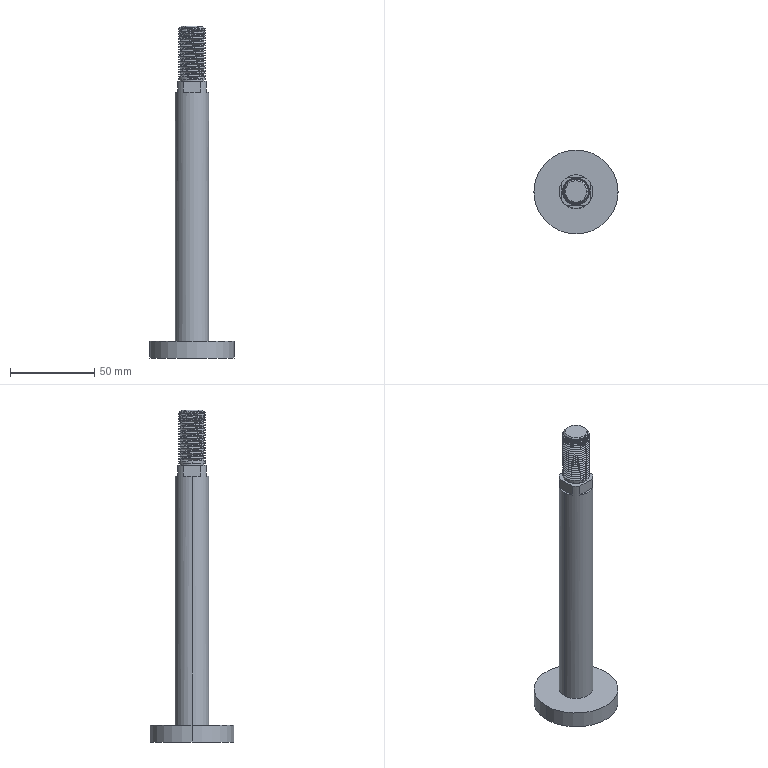Part | STEP file | 1 solid | 65 faces | box 50 x 50 x 197.5 mm | volume 73763 mm3 | cylinder 46 | plane 15 | cone 2 | spline 2 | commonest cylinder face diameters 16 x40 14 x2 20 x2 50 x2